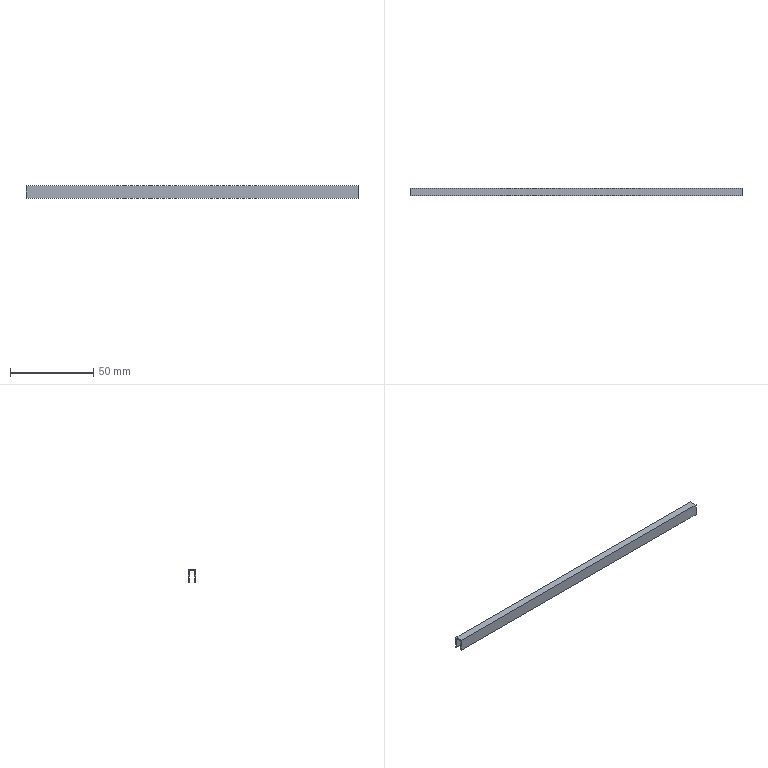Part | NX | features solid 2 | 1 solid | 10 faces | box 200 x 4.48 x 7.24 mm | volume 2131 mm3 | plane 10
STEP:
#1=CARTESIAN_POINT('',(255.,2180.06,-879.76));
#2=VERTEX_POINT('',#1);
#3=CARTESIAN_POINT('',(255.,2180.06,-887.));
#4=VERTEX_POINT('',#3);
#5=CARTESIAN_POINT('',(255.,2180.06,-879.76));
#6=DIRECTION('',(0.,0.,-1.));
#7=VECTOR('',#6,1000.);
#8=LINE('',#5,#7);
#9=EDGE_CURVE('',#2,#4,#8,.T.);
#10=ORIENTED_EDGE('',*,*,#9,.F.);
#11=CARTESIAN_POINT('',(55.,2180.06,-879.76));
#12=VERTEX_POINT('',#11);
#13=CARTESIAN_POINT('',(55.,2180.06,-879.76));
#14=DIRECTION('',(1.,0.,0.));
#15=VECTOR('',#14,1000.);
#16=LINE('',#13,#15);
#17=EDGE_CURVE('',#12,#2,#16,.T.);
#18=ORIENTED_EDGE('',*,*,#17,.F.);
#19=CARTESIAN_POINT('',(55.,2180.06,-887.));
#20=VERTEX_POINT('',#19);
#21=CARTESIAN_POINT('',(55.,2180.06,-879.76));
#22=DIRECTION('',(0.,0.,-1.));
#23=VECTOR('',#22,1000.);
#24=LINE('',#21,#23);
#25=EDGE_CURVE('',#12,#20,#24,.T.);
#26=ORIENTED_EDGE('',*,*,#25,.T.);
#27=CARTESIAN_POINT('',(255.,2180.06,-887.));
#28=DIRECTION('',(-1.,0.,0.));
#29=VECTOR('',#28,1000.);
#30=LINE('',#27,#29);
#31=EDGE_CURVE('',#4,#20,#30,.T.);
#32=ORIENTED_EDGE('',*,*,#31,.F.);
#33=EDGE_LOOP('',(#10,#18,#26,#32));
#34=FACE_BOUND('',#33,.T.);
#35=CARTESIAN_POINT('',(262.281,2180.06,-881.26));
#36=DIRECTION('',(0.,1.,0.));
#37=DIRECTION('',(0.,0.,1.));
#38=AXIS2_PLACEMENT_3D('',#35,#36,#37);
#39=PLANE('',#38);
#40=ADVANCED_FACE('',(#34),#39,.F.);
#41=CARTESIAN_POINT('',(255.,2180.66,-887.));
#42=VERTEX_POINT('',#41);
#43=CARTESIAN_POINT('',(255.,2180.06,-887.));
#44=DIRECTION('',(0.,1.,0.));
#45=VECTOR('',#44,1000.);
#46=LINE('',#43,#45);
#47=EDGE_CURVE('',#4,#42,#46,.T.);
#48=ORIENTED_EDGE('',*,*,#47,.F.);
#49=ORIENTED_EDGE('',*,*,#31,.T.);
#50=CARTESIAN_POINT('',(55.,2180.66,-887.));
#51=VERTEX_POINT('',#50);
#52=CARTESIAN_POINT('',(55.,2180.06,-887.));
#53=DIRECTION('',(0.,1.,0.));
#54=VECTOR('',#53,1000.);
#55=LINE('',#52,#54);
#56=EDGE_CURVE('',#20,#51,#55,.T.);
#57=ORIENTED_EDGE('',*,*,#56,.T.);
#58=CARTESIAN_POINT('',(55.,2180.66,-887.));
#59=DIRECTION('',(1.,0.,0.));
#60=VECTOR('',#59,1000.);
#61=LINE('',#58,#60);
#62=EDGE_CURVE('',#51,#42,#61,.T.);
#63=ORIENTED_EDGE('',*,*,#62,.T.);
#64=EDGE_LOOP('',(#48,#49,#57,#63));
#65=FACE_BOUND('',#64,.T.);
#66=CARTESIAN_POINT('',(262.281,2180.06,-887.));
#67=DIRECTION('',(0.,0.,1.));
#68=DIRECTION('',(0.,-1.,0.));
#69=AXIS2_PLACEMENT_3D('',#66,#67,#68);
#70=PLANE('',#69);
#71=ADVANCED_FACE('',(#65),#70,.F.);
#72=CARTESIAN_POINT('',(255.,2180.66,-880.36));
#73=VERTEX_POINT('',#72);
#74=CARTESIAN_POINT('',(255.,2180.66,-880.36));
#75=DIRECTION('',(0.,0.,-1.));
#76=VECTOR('',#75,1000.);
#77=LINE('',#74,#76);
#78=EDGE_CURVE('',#73,#42,#77,.T.);
#79=ORIENTED_EDGE('',*,*,#78,.T.);
#80=ORIENTED_EDGE('',*,*,#62,.F.);
#81=CARTESIAN_POINT('',(55.,2180.66,-880.36));
#82=VERTEX_POINT('',#81);
#83=CARTESIAN_POINT('',(55.,2180.66,-887.));
#84=DIRECTION('',(0.,0.,1.));
#85=VECTOR('',#84,1000.);
#86=LINE('',#83,#85);
#87=EDGE_CURVE('',#51,#82,#86,.T.);
#88=ORIENTED_EDGE('',*,*,#87,.T.);
#89=CARTESIAN_POINT('',(55.,2180.66,-880.36));
#90=DIRECTION('',(1.,0.,0.));
#91=VECTOR('',#90,1000.);
#92=LINE('',#89,#91);
#93=EDGE_CURVE('',#82,#73,#92,.T.);
#94=ORIENTED_EDGE('',*,*,#93,.T.);
#95=EDGE_LOOP('',(#79,#80,#88,#94));
#96=FACE_BOUND('',#95,.T.);
#97=CARTESIAN_POINT('',(262.281,2180.66,-881.26));
#98=DIRECTION('',(0.,1.,0.));
#99=DIRECTION('',(0.,0.,1.));
#100=AXIS2_PLACEMENT_3D('',#97,#98,#99);
#101=PLANE('',#100);
#102=ADVANCED_FACE('',(#96),#101,.T.);
#103=CARTESIAN_POINT('',(255.,2183.94,-880.36));
#104=VERTEX_POINT('',#103);
#105=CARTESIAN_POINT('',(255.,2183.94,-880.36));
#106=DIRECTION('',(0.,-1.,0.));
#107=VECTOR('',#106,1000.);
#108=LINE('',#105,#107);
#109=EDGE_CURVE('',#104,#73,#108,.T.);
#110=ORIENTED_EDGE('',*,*,#109,.T.);
#111=ORIENTED_EDGE('',*,*,#93,.F.);
#112=CARTESIAN_POINT('',(55.,2183.94,-880.36));
#113=VERTEX_POINT('',#112);
#114=CARTESIAN_POINT('',(55.,2180.66,-880.36));
#115=DIRECTION('',(0.,1.,0.));
#116=VECTOR('',#115,1000.);
#117=LINE('',#114,#116);
#118=EDGE_CURVE('',#82,#113,#117,.T.);
#119=ORIENTED_EDGE('',*,*,#118,.T.);
#120=CARTESIAN_POINT('',(55.,2183.94,-880.36));
#121=DIRECTION('',(1.,0.,0.));
#122=VECTOR('',#121,1000.);
#123=LINE('',#120,#122);
#124=EDGE_CURVE('',#113,#104,#123,.T.);
#125=ORIENTED_EDGE('',*,*,#124,.T.);
#126=EDGE_LOOP('',(#110,#111,#119,#125));
#127=FACE_BOUND('',#126,.T.);
#128=CARTESIAN_POINT('',(262.281,2184.54,-880.36));
#129=DIRECTION('',(0.,0.,-1.));
#130=DIRECTION('',(0.,1.,0.));
#131=AXIS2_PLACEMENT_3D('',#128,#129,#130);
#132=PLANE('',#131);
#133=ADVANCED_FACE('',(#127),#132,.T.);
#134=CARTESIAN_POINT('',(255.,2183.94,-887.));
#135=VERTEX_POINT('',#134);
#136=CARTESIAN_POINT('',(255.,2183.94,-887.));
#137=DIRECTION('',(0.,0.,1.));
#138=VECTOR('',#137,1000.);
#139=LINE('',#136,#138);
#140=EDGE_CURVE('',#135,#104,#139,.T.);
#141=ORIENTED_EDGE('',*,*,#140,.T.);
#142=ORIENTED_EDGE('',*,*,#124,.F.);
#143=CARTESIAN_POINT('',(55.,2183.94,-887.));
#144=VERTEX_POINT('',#143);
#145=CARTESIAN_POINT('',(55.,2183.94,-880.36));
#146=DIRECTION('',(0.,0.,-1.));
#147=VECTOR('',#146,1000.);
#148=LINE('',#145,#147);
#149=EDGE_CURVE('',#113,#144,#148,.T.);
#150=ORIENTED_EDGE('',*,*,#149,.T.);
#151=CARTESIAN_POINT('',(55.,2183.94,-887.));
#152=DIRECTION('',(1.,0.,0.));
#153=VECTOR('',#152,1000.);
#154=LINE('',#151,#153);
#155=EDGE_CURVE('',#144,#135,#154,.T.);
#156=ORIENTED_EDGE('',*,*,#155,.T.);
#157=EDGE_LOOP('',(#141,#142,#150,#156));
#158=FACE_BOUND('',#157,.T.);
#159=CARTESIAN_POINT('',(262.281,2183.94,-887.));
#160=DIRECTION('',(0.,-1.,0.));
#161=DIRECTION('',(-1.,0.,0.));
#162=AXIS2_PLACEMENT_3D('',#159,#160,#161);
#163=PLANE('',#162);
#164=ADVANCED_FACE('',(#158),#163,.T.);
#165=CARTESIAN_POINT('',(255.,2184.54,-887.));
#166=VERTEX_POINT('',#165);
#167=CARTESIAN_POINT('',(255.,2183.94,-887.));
#168=DIRECTION('',(0.,1.,0.));
#169=VECTOR('',#168,1000.);
#170=LINE('',#167,#169);
#171=EDGE_CURVE('',#135,#166,#170,.T.);
#172=ORIENTED_EDGE('',*,*,#171,.F.);
#173=ORIENTED_EDGE('',*,*,#155,.F.);
#174=CARTESIAN_POINT('',(55.,2184.54,-887.));
#175=VERTEX_POINT('',#174);
#176=CARTESIAN_POINT('',(55.,2183.94,-887.));
#177=DIRECTION('',(0.,1.,0.));
#178=VECTOR('',#177,1000.);
#179=LINE('',#176,#178);
#180=EDGE_CURVE('',#144,#175,#179,.T.);
#181=ORIENTED_EDGE('',*,*,#180,.T.);
#182=CARTESIAN_POINT('',(55.,2184.54,-887.));
#183=DIRECTION('',(1.,0.,0.));
#184=VECTOR('',#183,1000.);
#185=LINE('',#182,#184);
#186=EDGE_CURVE('',#175,#166,#185,.T.);
#187=ORIENTED_EDGE('',*,*,#186,.T.);
#188=EDGE_LOOP('',(#172,#173,#181,#187));
#189=FACE_BOUND('',#188,.T.);
#190=CARTESIAN_POINT('',(262.281,2183.94,-887.));
#191=DIRECTION('',(0.,0.,1.));
#192=DIRECTION('',(1.,0.,0.));
#193=AXIS2_PLACEMENT_3D('',#190,#191,#192);
#194=PLANE('',#193);
#195=ADVANCED_FACE('',(#189),#194,.F.);
#196=CARTESIAN_POINT('',(255.,2184.54,-879.76));
#197=VERTEX_POINT('',#196);
#198=CARTESIAN_POINT('',(255.,2184.54,-887.));
#199=DIRECTION('',(0.,0.,1.));
#200=VECTOR('',#199,1000.);
#201=LINE('',#198,#200);
#202=EDGE_CURVE('',#166,#197,#201,.T.);
#203=ORIENTED_EDGE('',*,*,#202,.F.);
#204=ORIENTED_EDGE('',*,*,#186,.F.);
#205=CARTESIAN_POINT('',(55.,2184.54,-879.76));
#206=VERTEX_POINT('',#205);
#207=CARTESIAN_POINT('',(55.,2184.54,-887.));
#208=DIRECTION('',(0.,0.,1.));
#209=VECTOR('',#208,1000.);
#210=LINE('',#207,#209);
#211=EDGE_CURVE('',#175,#206,#210,.T.);
#212=ORIENTED_EDGE('',*,*,#211,.T.);
#213=CARTESIAN_POINT('',(55.,2184.54,-879.76));
#214=DIRECTION('',(1.,0.,0.));
#215=VECTOR('',#214,1000.);
#216=LINE('',#213,#215);
#217=EDGE_CURVE('',#206,#197,#216,.T.);
#218=ORIENTED_EDGE('',*,*,#217,.T.);
#219=EDGE_LOOP('',(#203,#204,#212,#218));
#220=FACE_BOUND('',#219,.T.);
#221=CARTESIAN_POINT('',(262.281,2184.54,-887.));
#222=DIRECTION('',(0.,-1.,0.));
#223=DIRECTION('',(-1.,0.,0.));
#224=AXIS2_PLACEMENT_3D('',#221,#222,#223);
#225=PLANE('',#224);
#226=ADVANCED_FACE('',(#220),#225,.F.);
#227=CARTESIAN_POINT('',(255.,2184.54,-879.76));
#228=DIRECTION('',(0.,-1.,0.));
#229=VECTOR('',#228,1000.);
#230=LINE('',#227,#229);
#231=EDGE_CURVE('',#197,#2,#230,.T.);
#232=ORIENTED_EDGE('',*,*,#231,.F.);
#233=ORIENTED_EDGE('',*,*,#217,.F.);
#234=CARTESIAN_POINT('',(55.,2184.54,-879.76));
#235=DIRECTION('',(0.,-1.,0.));
#236=VECTOR('',#235,1000.);
#237=LINE('',#234,#236);
#238=EDGE_CURVE('',#206,#12,#237,.T.);
#239=ORIENTED_EDGE('',*,*,#238,.T.);
#240=ORIENTED_EDGE('',*,*,#17,.T.);
#241=EDGE_LOOP('',(#232,#233,#239,#240));
#242=FACE_BOUND('',#241,.T.);
#243=CARTESIAN_POINT('',(262.281,2184.54,-879.76));
#244=DIRECTION('',(0.,0.,-1.));
#245=DIRECTION('',(0.,1.,0.));
#246=AXIS2_PLACEMENT_3D('',#243,#244,#245);
#247=PLANE('',#246);
#248=ADVANCED_FACE('',(#242),#247,.F.);
#249=ORIENTED_EDGE('',*,*,#238,.F.);
#250=ORIENTED_EDGE('',*,*,#211,.F.);
#251=ORIENTED_EDGE('',*,*,#180,.F.);
#252=ORIENTED_EDGE('',*,*,#149,.F.);
#253=ORIENTED_EDGE('',*,*,#118,.F.);
#254=ORIENTED_EDGE('',*,*,#87,.F.);
#255=ORIENTED_EDGE('',*,*,#56,.F.);
#256=ORIENTED_EDGE('',*,*,#25,.F.);
#257=EDGE_LOOP('',(#249,#250,#251,#252,#253,#254,#255,#256));
#258=FACE_BOUND('',#257,.T.);
#259=CARTESIAN_POINT('',(55.,2182.3,-880.));
#260=DIRECTION('',(-1.,0.,0.));
#261=DIRECTION('',(0.,1.,0.));
#262=AXIS2_PLACEMENT_3D('',#259,#260,#261);
#263=PLANE('',#262);
#264=ADVANCED_FACE('',(#258),#263,.T.);
#265=ORIENTED_EDGE('',*,*,#109,.F.);
#266=ORIENTED_EDGE('',*,*,#140,.F.);
#267=ORIENTED_EDGE('',*,*,#171,.T.);
#268=ORIENTED_EDGE('',*,*,#202,.T.);
#269=ORIENTED_EDGE('',*,*,#231,.T.);
#270=ORIENTED_EDGE('',*,*,#9,.T.);
#271=ORIENTED_EDGE('',*,*,#47,.T.);
#272=ORIENTED_EDGE('',*,*,#78,.F.);
#273=EDGE_LOOP('',(#265,#266,#267,#268,#269,#270,#271,#272));
#274=FACE_BOUND('',#273,.T.);
#275=CARTESIAN_POINT('',(255.,2182.3,-880.));
#276=DIRECTION('',(1.,0.,0.));
#277=DIRECTION('',(0.,-1.,0.));
#278=AXIS2_PLACEMENT_3D('',#275,#276,#277);
#279=PLANE('',#278);
#280=ADVANCED_FACE('',(#274),#279,.T.);
#281=CLOSED_SHELL('',(#40,#71,#102,#133,#164,#195,#226,#248,#264,#280));
#282=MANIFOLD_SOLID_BREP('',#281);
#283=(LENGTH_UNIT()NAMED_UNIT(*)SI_UNIT(.MILLI.,.METRE.));
#284=UNCERTAINTY_MEASURE_WITH_UNIT(LENGTH_MEASURE(0.00001),#283,'','');
#285=(NAMED_UNIT(*)PLANE_ANGLE_UNIT()SI_UNIT($,.RADIAN.));
#286=(NAMED_UNIT(*)SI_UNIT($,.STERADIAN.)SOLID_ANGLE_UNIT());
#287=(GEOMETRIC_REPRESENTATION_CONTEXT(3)GLOBAL_UNCERTAINTY_ASSIGNED_CONTEXT((#284))GLOBAL_UNIT_ASSIGNED_CONTEXT((#283,#285,#286))REPRESENTATION_CONTEXT('',''));
#288=ADVANCED_BREP_SHAPE_REPRESENTATION('',(#282),#287);